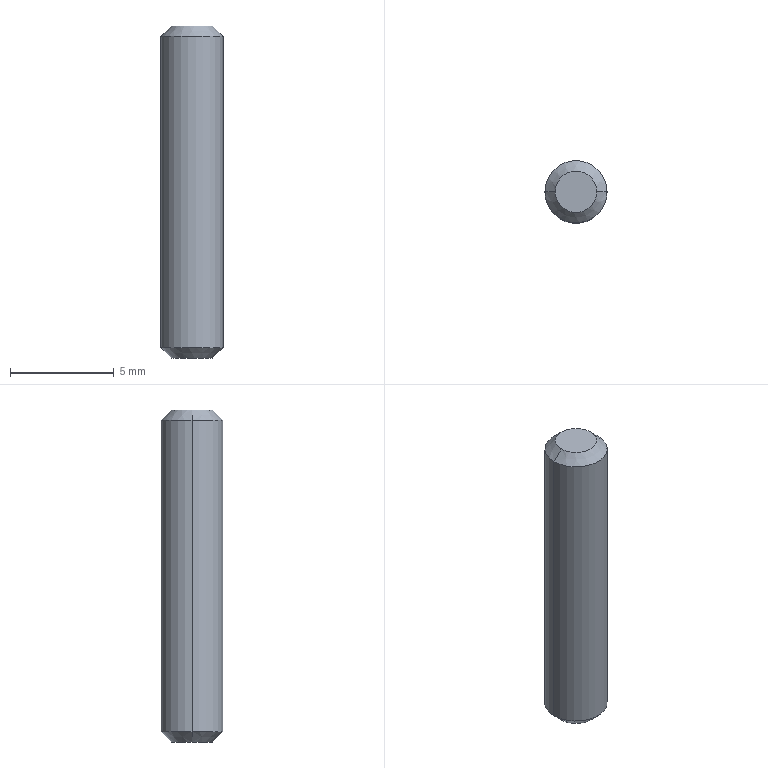Part | SolidWorks | features BaseBody 1 | 1 solid | 8 faces | box 3 x 3 x 16 mm | volume 111.003 mm3 | cone 4 | cylinder 2 | plane 2 | commonest cylinder face diameters 3 x2
STEP:
#1=CARTESIAN_POINT('',(1.5,0.,0.5));
#2=VERTEX_POINT('',#1);
#3=CARTESIAN_POINT('',(-1.5,0.,0.5));
#4=VERTEX_POINT('',#3);
#5=CARTESIAN_POINT('',(0.,0.,0.5));
#6=DIRECTION('',(0.,0.,1.));
#7=DIRECTION('',(1.,0.,0.));
#8=AXIS2_PLACEMENT_3D('',#5,#6,#7);
#9=CIRCLE('',#8,1.5);
#10=EDGE_CURVE('',#2,#4,#9,.T.);
#11=ORIENTED_EDGE('',*,*,#10,.T.);
#12=CARTESIAN_POINT('',(-1.5,0.,15.5));
#13=VERTEX_POINT('',#12);
#14=CARTESIAN_POINT('',(-1.5,0.,0.));
#15=DIRECTION('',(0.,0.,1.));
#16=VECTOR('',#15,1000.);
#17=LINE('',#14,#16);
#18=EDGE_CURVE('',#4,#13,#17,.T.);
#19=ORIENTED_EDGE('',*,*,#18,.T.);
#20=CARTESIAN_POINT('',(1.5,0.,15.5));
#21=VERTEX_POINT('',#20);
#22=CARTESIAN_POINT('',(0.,0.,15.5));
#23=DIRECTION('',(0.,0.,-1.));
#24=DIRECTION('',(1.,0.,0.));
#25=AXIS2_PLACEMENT_3D('',#22,#23,#24);
#26=CIRCLE('',#25,1.5);
#27=EDGE_CURVE('',#13,#21,#26,.T.);
#28=ORIENTED_EDGE('',*,*,#27,.T.);
#29=CARTESIAN_POINT('',(1.5,0.,0.));
#30=DIRECTION('',(0.,0.,1.));
#31=VECTOR('',#30,1000.);
#32=LINE('',#29,#31);
#33=EDGE_CURVE('',#2,#21,#32,.T.);
#34=ORIENTED_EDGE('',*,*,#33,.F.);
#35=EDGE_LOOP('',(#11,#19,#28,#34));
#36=FACE_OUTER_BOUND('',#35,.T.);
#37=CARTESIAN_POINT('',(0.,0.,0.));
#38=DIRECTION('',(0.,0.,1.));
#39=DIRECTION('',(1.,0.,0.));
#40=AXIS2_PLACEMENT_3D('',#37,#38,#39);
#41=CYLINDRICAL_SURFACE('',#40,1.5);
#42=ADVANCED_FACE('',(#36),#41,.T.);
#43=CARTESIAN_POINT('',(1.,0.,0.));
#44=VERTEX_POINT('',#43);
#45=CARTESIAN_POINT('',(-1.,0.,0.));
#46=VERTEX_POINT('',#45);
#47=CARTESIAN_POINT('',(0.,0.,0.));
#48=DIRECTION('',(0.,0.,1.));
#49=DIRECTION('',(1.,0.,0.));
#50=AXIS2_PLACEMENT_3D('',#47,#48,#49);
#51=CIRCLE('',#50,1.);
#52=EDGE_CURVE('',#44,#46,#51,.T.);
#53=ORIENTED_EDGE('',*,*,#52,.T.);
#54=CARTESIAN_POINT('',(-1.5,0.,0.5));
#55=DIRECTION('',(-0.7071,0.,0.7071));
#56=VECTOR('',#55,1000.);
#57=LINE('',#54,#56);
#58=EDGE_CURVE('',#46,#4,#57,.T.);
#59=ORIENTED_EDGE('',*,*,#58,.T.);
#60=ORIENTED_EDGE('',*,*,#10,.F.);
#61=CARTESIAN_POINT('',(1.5,0.,0.5));
#62=DIRECTION('',(0.7071,0.,0.7071));
#63=VECTOR('',#62,1000.);
#64=LINE('',#61,#63);
#65=EDGE_CURVE('',#44,#2,#64,.T.);
#66=ORIENTED_EDGE('',*,*,#65,.F.);
#67=EDGE_LOOP('',(#53,#59,#60,#66));
#68=FACE_OUTER_BOUND('',#67,.T.);
#69=CARTESIAN_POINT('',(0.,0.,0.5));
#70=DIRECTION('',(0.,0.,1.));
#71=DIRECTION('',(1.,0.,0.));
#72=AXIS2_PLACEMENT_3D('',#69,#70,#71);
#73=CONICAL_SURFACE('',#72,1.5,0.7854);
#74=ADVANCED_FACE('',(#68),#73,.T.);
#75=CARTESIAN_POINT('',(-1.,0.,16.));
#76=VERTEX_POINT('',#75);
#77=CARTESIAN_POINT('',(1.,0.,16.));
#78=VERTEX_POINT('',#77);
#79=CARTESIAN_POINT('',(0.,0.,16.));
#80=DIRECTION('',(0.,0.,-1.));
#81=DIRECTION('',(-1.,0.,0.));
#82=AXIS2_PLACEMENT_3D('',#79,#80,#81);
#83=CIRCLE('',#82,1.);
#84=EDGE_CURVE('',#76,#78,#83,.T.);
#85=ORIENTED_EDGE('',*,*,#84,.T.);
#86=CARTESIAN_POINT('',(1.5,0.,15.5));
#87=DIRECTION('',(0.7071,0.,-0.7071));
#88=VECTOR('',#87,1000.);
#89=LINE('',#86,#88);
#90=EDGE_CURVE('',#78,#21,#89,.T.);
#91=ORIENTED_EDGE('',*,*,#90,.T.);
#92=ORIENTED_EDGE('',*,*,#27,.F.);
#93=CARTESIAN_POINT('',(-1.5,0.,15.5));
#94=DIRECTION('',(-0.7071,0.,-0.7071));
#95=VECTOR('',#94,1000.);
#96=LINE('',#93,#95);
#97=EDGE_CURVE('',#76,#13,#96,.T.);
#98=ORIENTED_EDGE('',*,*,#97,.F.);
#99=EDGE_LOOP('',(#85,#91,#92,#98));
#100=FACE_OUTER_BOUND('',#99,.T.);
#101=CARTESIAN_POINT('',(0.,0.,15.5));
#102=DIRECTION('',(0.,0.,-1.));
#103=DIRECTION('',(-1.,0.,0.));
#104=AXIS2_PLACEMENT_3D('',#101,#102,#103);
#105=CONICAL_SURFACE('',#104,1.5,0.7854);
#106=ADVANCED_FACE('',(#100),#105,.T.);
#107=ORIENTED_EDGE('',*,*,#18,.F.);
#108=CARTESIAN_POINT('',(0.,0.,0.5));
#109=DIRECTION('',(0.,0.,1.));
#110=DIRECTION('',(1.,0.,0.));
#111=AXIS2_PLACEMENT_3D('',#108,#109,#110);
#112=CIRCLE('',#111,1.5);
#113=EDGE_CURVE('',#4,#2,#112,.T.);
#114=ORIENTED_EDGE('',*,*,#113,.T.);
#115=ORIENTED_EDGE('',*,*,#33,.T.);
#116=CARTESIAN_POINT('',(0.,0.,15.5));
#117=DIRECTION('',(0.,0.,-1.));
#118=DIRECTION('',(1.,0.,0.));
#119=AXIS2_PLACEMENT_3D('',#116,#117,#118);
#120=CIRCLE('',#119,1.5);
#121=EDGE_CURVE('',#21,#13,#120,.T.);
#122=ORIENTED_EDGE('',*,*,#121,.T.);
#123=EDGE_LOOP('',(#107,#114,#115,#122));
#124=FACE_OUTER_BOUND('',#123,.T.);
#125=CARTESIAN_POINT('',(0.,0.,0.));
#126=DIRECTION('',(0.,0.,1.));
#127=DIRECTION('',(1.,0.,0.));
#128=AXIS2_PLACEMENT_3D('',#125,#126,#127);
#129=CYLINDRICAL_SURFACE('',#128,1.5);
#130=ADVANCED_FACE('',(#124),#129,.T.);
#131=ORIENTED_EDGE('',*,*,#58,.F.);
#132=CARTESIAN_POINT('',(0.,0.,0.));
#133=DIRECTION('',(0.,0.,1.));
#134=DIRECTION('',(1.,0.,0.));
#135=AXIS2_PLACEMENT_3D('',#132,#133,#134);
#136=CIRCLE('',#135,1.);
#137=EDGE_CURVE('',#46,#44,#136,.T.);
#138=ORIENTED_EDGE('',*,*,#137,.T.);
#139=ORIENTED_EDGE('',*,*,#65,.T.);
#140=ORIENTED_EDGE('',*,*,#113,.F.);
#141=EDGE_LOOP('',(#131,#138,#139,#140));
#142=FACE_OUTER_BOUND('',#141,.T.);
#143=CARTESIAN_POINT('',(0.,0.,0.5));
#144=DIRECTION('',(0.,0.,1.));
#145=DIRECTION('',(1.,0.,0.));
#146=AXIS2_PLACEMENT_3D('',#143,#144,#145);
#147=CONICAL_SURFACE('',#146,1.5,0.7854);
#148=ADVANCED_FACE('',(#142),#147,.T.);
#149=ORIENTED_EDGE('',*,*,#90,.F.);
#150=CARTESIAN_POINT('',(0.,0.,16.));
#151=DIRECTION('',(0.,0.,-1.));
#152=DIRECTION('',(-1.,0.,0.));
#153=AXIS2_PLACEMENT_3D('',#150,#151,#152);
#154=CIRCLE('',#153,1.);
#155=EDGE_CURVE('',#78,#76,#154,.T.);
#156=ORIENTED_EDGE('',*,*,#155,.T.);
#157=ORIENTED_EDGE('',*,*,#97,.T.);
#158=ORIENTED_EDGE('',*,*,#121,.F.);
#159=EDGE_LOOP('',(#149,#156,#157,#158));
#160=FACE_OUTER_BOUND('',#159,.T.);
#161=CARTESIAN_POINT('',(0.,0.,15.5));
#162=DIRECTION('',(0.,0.,-1.));
#163=DIRECTION('',(-1.,0.,0.));
#164=AXIS2_PLACEMENT_3D('',#161,#162,#163);
#165=CONICAL_SURFACE('',#164,1.5,0.7854);
#166=ADVANCED_FACE('',(#160),#165,.T.);
#167=ORIENTED_EDGE('',*,*,#52,.F.);
#168=ORIENTED_EDGE('',*,*,#137,.F.);
#169=EDGE_LOOP('',(#167,#168));
#170=FACE_OUTER_BOUND('',#169,.T.);
#171=CARTESIAN_POINT('',(0.,0.,0.));
#172=DIRECTION('',(0.,0.,-1.));
#173=DIRECTION('',(-1.,0.,0.));
#174=AXIS2_PLACEMENT_3D('',#171,#172,#173);
#175=PLANE('',#174);
#176=ADVANCED_FACE('',(#170),#175,.T.);
#177=ORIENTED_EDGE('',*,*,#84,.F.);
#178=ORIENTED_EDGE('',*,*,#155,.F.);
#179=EDGE_LOOP('',(#177,#178));
#180=FACE_OUTER_BOUND('',#179,.T.);
#181=CARTESIAN_POINT('',(0.,0.,16.));
#182=DIRECTION('',(0.,0.,-1.));
#183=DIRECTION('',(-1.,0.,0.));
#184=AXIS2_PLACEMENT_3D('',#181,#182,#183);
#185=PLANE('',#184);
#186=ADVANCED_FACE('',(#180),#185,.F.);
#187=CLOSED_SHELL('',(#42,#74,#106,#130,#148,#166,#176,#186));
#188=MANIFOLD_SOLID_BREP('',#187);
#189=CARTESIAN_POINT('',(0.,0.,0.));
#190=DIRECTION('',(0.,0.,1.));
#191=DIRECTION('',(1.,0.,0.));
#192=AXIS2_PLACEMENT_3D('',#189,#190,#191);
#193=(LENGTH_UNIT()NAMED_UNIT(*)SI_UNIT(.MILLI.,.METRE.));
#194=UNCERTAINTY_MEASURE_WITH_UNIT(LENGTH_MEASURE(0.00001),#193,'','');
#195=(NAMED_UNIT(*)PLANE_ANGLE_UNIT()SI_UNIT($,.RADIAN.));
#196=(NAMED_UNIT(*)SI_UNIT($,.STERADIAN.)SOLID_ANGLE_UNIT());
#197=(GEOMETRIC_REPRESENTATION_CONTEXT(3)GLOBAL_UNCERTAINTY_ASSIGNED_CONTEXT((#194))GLOBAL_UNIT_ASSIGNED_CONTEXT((#193,#195,#196))REPRESENTATION_CONTEXT('',''));
#198=ADVANCED_BREP_SHAPE_REPRESENTATION('',(#188,#192),#197);